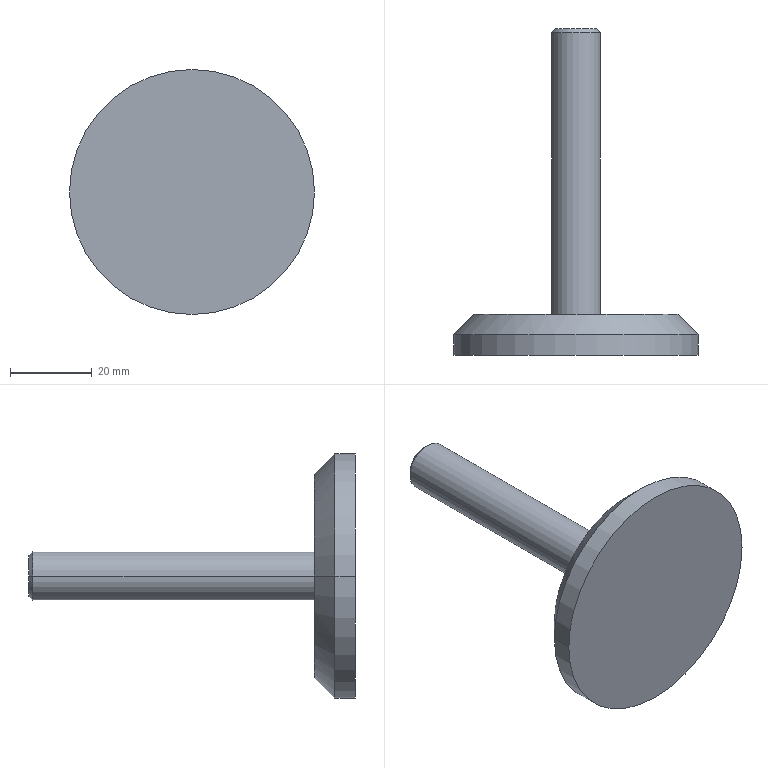Part | STEP file | Main support leg M12 for conveyor | 1 solid | 11 faces | box 60 x 80 x 60 mm | volume 33948 mm3 | cone 4 | cylinder 4 | plane 3 | commonest cylinder face diameters 12 x2 60 x2
STEP:
#1=CARTESIAN_POINT('',(-5.,80.,0.));
#2=VERTEX_POINT('',#1);
#3=CARTESIAN_POINT('',(5.,80.,0.));
#4=VERTEX_POINT('',#3);
#5=CARTESIAN_POINT('',(0.,80.,0.));
#6=DIRECTION('',(0.,1.,0.));
#7=DIRECTION('',(-1.,0.,0.));
#8=AXIS2_PLACEMENT_3D('',#5,#6,#7);
#9=CIRCLE('',#8,5.);
#10=EDGE_CURVE('',#2,#4,#9,.T.);
#11=ORIENTED_EDGE('',*,*,#10,.F.);
#12=CARTESIAN_POINT('',(-6.,79.,0.));
#13=VERTEX_POINT('',#12);
#14=CARTESIAN_POINT('',(-5.,80.,0.));
#15=DIRECTION('',(-0.7071,-0.7071,0.));
#16=VECTOR('',#15,1000.);
#17=LINE('',#14,#16);
#18=EDGE_CURVE('',#2,#13,#17,.T.);
#19=ORIENTED_EDGE('',*,*,#18,.T.);
#20=CARTESIAN_POINT('',(6.,79.,0.));
#21=VERTEX_POINT('',#20);
#22=CARTESIAN_POINT('',(0.,79.,0.));
#23=DIRECTION('',(0.,-1.,0.));
#24=DIRECTION('',(-1.,0.,0.));
#25=AXIS2_PLACEMENT_3D('',#22,#23,#24);
#26=CIRCLE('',#25,6.);
#27=EDGE_CURVE('',#21,#13,#26,.T.);
#28=ORIENTED_EDGE('',*,*,#27,.F.);
#29=CARTESIAN_POINT('',(5.,80.,0.));
#30=DIRECTION('',(0.7071,-0.7071,0.));
#31=VECTOR('',#30,1000.);
#32=LINE('',#29,#31);
#33=EDGE_CURVE('',#4,#21,#32,.T.);
#34=ORIENTED_EDGE('',*,*,#33,.F.);
#35=EDGE_LOOP('',(#11,#19,#28,#34));
#36=FACE_OUTER_BOUND('',#35,.T.);
#37=CARTESIAN_POINT('',(0.,80.,0.));
#38=DIRECTION('',(0.,-1.,0.));
#39=DIRECTION('',(1.,0.,0.));
#40=AXIS2_PLACEMENT_3D('',#37,#38,#39);
#41=CONICAL_SURFACE('',#40,5.,0.7854);
#42=ADVANCED_FACE('',(#36),#41,.T.);
#43=CARTESIAN_POINT('',(-6.,10.,0.));
#44=VERTEX_POINT('',#43);
#45=CARTESIAN_POINT('',(6.,10.,0.));
#46=VERTEX_POINT('',#45);
#47=CARTESIAN_POINT('',(0.,10.,0.));
#48=DIRECTION('',(0.,1.,0.));
#49=DIRECTION('',(-1.,0.,0.));
#50=AXIS2_PLACEMENT_3D('',#47,#48,#49);
#51=CIRCLE('',#50,6.);
#52=EDGE_CURVE('',#44,#46,#51,.T.);
#53=ORIENTED_EDGE('',*,*,#52,.T.);
#54=CARTESIAN_POINT('',(6.,80.,0.));
#55=DIRECTION('',(0.,1.,0.));
#56=VECTOR('',#55,1000.);
#57=LINE('',#54,#56);
#58=EDGE_CURVE('',#46,#21,#57,.T.);
#59=ORIENTED_EDGE('',*,*,#58,.T.);
#60=ORIENTED_EDGE('',*,*,#27,.T.);
#61=CARTESIAN_POINT('',(-6.,80.,0.));
#62=DIRECTION('',(0.,1.,0.));
#63=VECTOR('',#62,1000.);
#64=LINE('',#61,#63);
#65=EDGE_CURVE('',#44,#13,#64,.T.);
#66=ORIENTED_EDGE('',*,*,#65,.F.);
#67=EDGE_LOOP('',(#53,#59,#60,#66));
#68=FACE_OUTER_BOUND('',#67,.T.);
#69=CARTESIAN_POINT('',(0.,80.,0.));
#70=DIRECTION('',(0.,1.,0.));
#71=DIRECTION('',(-1.,0.,0.));
#72=AXIS2_PLACEMENT_3D('',#69,#70,#71);
#73=CYLINDRICAL_SURFACE('',#72,6.);
#74=ADVANCED_FACE('',(#68),#73,.T.);
#75=CARTESIAN_POINT('',(-25.,10.,0.));
#76=VERTEX_POINT('',#75);
#77=CARTESIAN_POINT('',(25.,10.,0.));
#78=VERTEX_POINT('',#77);
#79=CARTESIAN_POINT('',(0.,10.,0.));
#80=DIRECTION('',(0.,1.,0.));
#81=DIRECTION('',(-1.,0.,0.));
#82=AXIS2_PLACEMENT_3D('',#79,#80,#81);
#83=CIRCLE('',#82,25.);
#84=EDGE_CURVE('',#76,#78,#83,.T.);
#85=ORIENTED_EDGE('',*,*,#84,.F.);
#86=CARTESIAN_POINT('',(-30.,5.,0.));
#87=VERTEX_POINT('',#86);
#88=CARTESIAN_POINT('',(-25.,10.,0.));
#89=DIRECTION('',(-0.7071,-0.7071,0.));
#90=VECTOR('',#89,1000.);
#91=LINE('',#88,#90);
#92=EDGE_CURVE('',#76,#87,#91,.T.);
#93=ORIENTED_EDGE('',*,*,#92,.T.);
#94=CARTESIAN_POINT('',(30.,5.,0.));
#95=VERTEX_POINT('',#94);
#96=CARTESIAN_POINT('',(0.,5.,0.));
#97=DIRECTION('',(0.,1.,0.));
#98=DIRECTION('',(-1.,0.,0.));
#99=AXIS2_PLACEMENT_3D('',#96,#97,#98);
#100=CIRCLE('',#99,30.);
#101=EDGE_CURVE('',#87,#95,#100,.T.);
#102=ORIENTED_EDGE('',*,*,#101,.T.);
#103=CARTESIAN_POINT('',(25.,10.,0.));
#104=DIRECTION('',(0.7071,-0.7071,0.));
#105=VECTOR('',#104,1000.);
#106=LINE('',#103,#105);
#107=EDGE_CURVE('',#78,#95,#106,.T.);
#108=ORIENTED_EDGE('',*,*,#107,.F.);
#109=EDGE_LOOP('',(#85,#93,#102,#108));
#110=FACE_OUTER_BOUND('',#109,.T.);
#111=CARTESIAN_POINT('',(0.,10.,0.));
#112=DIRECTION('',(0.,-1.,0.));
#113=DIRECTION('',(1.,0.,0.));
#114=AXIS2_PLACEMENT_3D('',#111,#112,#113);
#115=CONICAL_SURFACE('',#114,25.,0.7854);
#116=ADVANCED_FACE('',(#110),#115,.T.);
#117=CARTESIAN_POINT('',(-30.,0.,0.));
#118=VERTEX_POINT('',#117);
#119=CARTESIAN_POINT('',(30.,0.,0.));
#120=VERTEX_POINT('',#119);
#121=CARTESIAN_POINT('',(0.,0.,0.));
#122=DIRECTION('',(0.,1.,0.));
#123=DIRECTION('',(-1.,0.,0.));
#124=AXIS2_PLACEMENT_3D('',#121,#122,#123);
#125=CIRCLE('',#124,30.);
#126=EDGE_CURVE('',#118,#120,#125,.T.);
#127=ORIENTED_EDGE('',*,*,#126,.T.);
#128=CARTESIAN_POINT('',(30.,80.,0.));
#129=DIRECTION('',(0.,1.,0.));
#130=VECTOR('',#129,1000.);
#131=LINE('',#128,#130);
#132=EDGE_CURVE('',#120,#95,#131,.T.);
#133=ORIENTED_EDGE('',*,*,#132,.T.);
#134=ORIENTED_EDGE('',*,*,#101,.F.);
#135=CARTESIAN_POINT('',(-30.,80.,0.));
#136=DIRECTION('',(0.,1.,0.));
#137=VECTOR('',#136,1000.);
#138=LINE('',#135,#137);
#139=EDGE_CURVE('',#118,#87,#138,.T.);
#140=ORIENTED_EDGE('',*,*,#139,.F.);
#141=EDGE_LOOP('',(#127,#133,#134,#140));
#142=FACE_OUTER_BOUND('',#141,.T.);
#143=CARTESIAN_POINT('',(0.,80.,0.));
#144=DIRECTION('',(0.,1.,0.));
#145=DIRECTION('',(-1.,0.,0.));
#146=AXIS2_PLACEMENT_3D('',#143,#144,#145);
#147=CYLINDRICAL_SURFACE('',#146,30.);
#148=ADVANCED_FACE('',(#142),#147,.T.);
#149=ORIENTED_EDGE('',*,*,#126,.F.);
#150=CARTESIAN_POINT('',(0.,0.,0.));
#151=DIRECTION('',(0.,1.,0.));
#152=DIRECTION('',(-1.,0.,0.));
#153=AXIS2_PLACEMENT_3D('',#150,#151,#152);
#154=CIRCLE('',#153,30.);
#155=EDGE_CURVE('',#120,#118,#154,.T.);
#156=ORIENTED_EDGE('',*,*,#155,.F.);
#157=EDGE_LOOP('',(#149,#156));
#158=FACE_OUTER_BOUND('',#157,.T.);
#159=CARTESIAN_POINT('',(0.,0.,0.));
#160=DIRECTION('',(0.,-1.,0.));
#161=DIRECTION('',(1.,0.,0.));
#162=AXIS2_PLACEMENT_3D('',#159,#160,#161);
#163=PLANE('',#162);
#164=ADVANCED_FACE('',(#158),#163,.T.);
#165=ORIENTED_EDGE('',*,*,#132,.F.);
#166=ORIENTED_EDGE('',*,*,#155,.T.);
#167=ORIENTED_EDGE('',*,*,#139,.T.);
#168=CARTESIAN_POINT('',(0.,5.,0.));
#169=DIRECTION('',(0.,1.,0.));
#170=DIRECTION('',(-1.,0.,0.));
#171=AXIS2_PLACEMENT_3D('',#168,#169,#170);
#172=CIRCLE('',#171,30.);
#173=EDGE_CURVE('',#95,#87,#172,.T.);
#174=ORIENTED_EDGE('',*,*,#173,.F.);
#175=EDGE_LOOP('',(#165,#166,#167,#174));
#176=FACE_OUTER_BOUND('',#175,.T.);
#177=CARTESIAN_POINT('',(0.,80.,0.));
#178=DIRECTION('',(0.,1.,0.));
#179=DIRECTION('',(-1.,0.,0.));
#180=AXIS2_PLACEMENT_3D('',#177,#178,#179);
#181=CYLINDRICAL_SURFACE('',#180,30.);
#182=ADVANCED_FACE('',(#176),#181,.T.);
#183=ORIENTED_EDGE('',*,*,#92,.F.);
#184=CARTESIAN_POINT('',(0.,10.,0.));
#185=DIRECTION('',(0.,1.,0.));
#186=DIRECTION('',(-1.,0.,0.));
#187=AXIS2_PLACEMENT_3D('',#184,#185,#186);
#188=CIRCLE('',#187,25.);
#189=EDGE_CURVE('',#78,#76,#188,.T.);
#190=ORIENTED_EDGE('',*,*,#189,.F.);
#191=ORIENTED_EDGE('',*,*,#107,.T.);
#192=ORIENTED_EDGE('',*,*,#173,.T.);
#193=EDGE_LOOP('',(#183,#190,#191,#192));
#194=FACE_OUTER_BOUND('',#193,.T.);
#195=CARTESIAN_POINT('',(0.,10.,0.));
#196=DIRECTION('',(0.,-1.,0.));
#197=DIRECTION('',(1.,0.,0.));
#198=AXIS2_PLACEMENT_3D('',#195,#196,#197);
#199=CONICAL_SURFACE('',#198,25.,0.7854);
#200=ADVANCED_FACE('',(#194),#199,.T.);
#201=ORIENTED_EDGE('',*,*,#189,.T.);
#202=ORIENTED_EDGE('',*,*,#84,.T.);
#203=EDGE_LOOP('',(#201,#202));
#204=FACE_OUTER_BOUND('',#203,.T.);
#205=ORIENTED_EDGE('',*,*,#52,.F.);
#206=CARTESIAN_POINT('',(0.,10.,0.));
#207=DIRECTION('',(0.,1.,0.));
#208=DIRECTION('',(-1.,0.,0.));
#209=AXIS2_PLACEMENT_3D('',#206,#207,#208);
#210=CIRCLE('',#209,6.);
#211=EDGE_CURVE('',#46,#44,#210,.T.);
#212=ORIENTED_EDGE('',*,*,#211,.F.);
#213=EDGE_LOOP('',(#205,#212));
#214=FACE_BOUND('',#213,.T.);
#215=CARTESIAN_POINT('',(-25.,10.,0.));
#216=DIRECTION('',(0.,1.,0.));
#217=DIRECTION('',(-1.,0.,0.));
#218=AXIS2_PLACEMENT_3D('',#215,#216,#217);
#219=PLANE('',#218);
#220=ADVANCED_FACE('',(#204,#214),#219,.T.);
#221=ORIENTED_EDGE('',*,*,#58,.F.);
#222=ORIENTED_EDGE('',*,*,#211,.T.);
#223=ORIENTED_EDGE('',*,*,#65,.T.);
#224=CARTESIAN_POINT('',(0.,79.,0.));
#225=DIRECTION('',(0.,-1.,0.));
#226=DIRECTION('',(-1.,0.,0.));
#227=AXIS2_PLACEMENT_3D('',#224,#225,#226);
#228=CIRCLE('',#227,6.);
#229=EDGE_CURVE('',#13,#21,#228,.T.);
#230=ORIENTED_EDGE('',*,*,#229,.T.);
#231=EDGE_LOOP('',(#221,#222,#223,#230));
#232=FACE_OUTER_BOUND('',#231,.T.);
#233=CARTESIAN_POINT('',(0.,80.,0.));
#234=DIRECTION('',(0.,1.,0.));
#235=DIRECTION('',(-1.,0.,0.));
#236=AXIS2_PLACEMENT_3D('',#233,#234,#235);
#237=CYLINDRICAL_SURFACE('',#236,6.);
#238=ADVANCED_FACE('',(#232),#237,.T.);
#239=CARTESIAN_POINT('',(0.,80.,0.));
#240=DIRECTION('',(0.,1.,0.));
#241=DIRECTION('',(-1.,0.,0.));
#242=AXIS2_PLACEMENT_3D('',#239,#240,#241);
#243=CIRCLE('',#242,5.);
#244=EDGE_CURVE('',#4,#2,#243,.T.);
#245=ORIENTED_EDGE('',*,*,#244,.T.);
#246=ORIENTED_EDGE('',*,*,#10,.T.);
#247=EDGE_LOOP('',(#245,#246));
#248=FACE_OUTER_BOUND('',#247,.T.);
#249=CARTESIAN_POINT('',(-6.,80.,0.));
#250=DIRECTION('',(0.,1.,0.));
#251=DIRECTION('',(-1.,0.,0.));
#252=AXIS2_PLACEMENT_3D('',#249,#250,#251);
#253=PLANE('',#252);
#254=ADVANCED_FACE('',(#248),#253,.T.);
#255=ORIENTED_EDGE('',*,*,#18,.F.);
#256=ORIENTED_EDGE('',*,*,#244,.F.);
#257=ORIENTED_EDGE('',*,*,#33,.T.);
#258=ORIENTED_EDGE('',*,*,#229,.F.);
#259=EDGE_LOOP('',(#255,#256,#257,#258));
#260=FACE_OUTER_BOUND('',#259,.T.);
#261=CARTESIAN_POINT('',(0.,80.,0.));
#262=DIRECTION('',(0.,-1.,0.));
#263=DIRECTION('',(1.,0.,0.));
#264=AXIS2_PLACEMENT_3D('',#261,#262,#263);
#265=CONICAL_SURFACE('',#264,5.,0.7854);
#266=ADVANCED_FACE('',(#260),#265,.T.);
#267=CLOSED_SHELL('',(#42,#74,#116,#148,#164,#182,#200,#220,#238,#254,#266));
#268=MANIFOLD_SOLID_BREP('',#267);
#269=CARTESIAN_POINT('',(0.,0.,0.));
#270=DIRECTION('',(0.,0.,1.));
#271=DIRECTION('',(1.,0.,0.));
#272=AXIS2_PLACEMENT_3D('',#269,#270,#271);
#273=(LENGTH_UNIT()NAMED_UNIT(*)SI_UNIT(.MILLI.,.METRE.));
#274=UNCERTAINTY_MEASURE_WITH_UNIT(LENGTH_MEASURE(0.00001),#273,'','');
#275=(NAMED_UNIT(*)PLANE_ANGLE_UNIT()SI_UNIT($,.RADIAN.));
#276=(NAMED_UNIT(*)SI_UNIT($,.STERADIAN.)SOLID_ANGLE_UNIT());
#277=(GEOMETRIC_REPRESENTATION_CONTEXT(3)GLOBAL_UNCERTAINTY_ASSIGNED_CONTEXT((#274))GLOBAL_UNIT_ASSIGNED_CONTEXT((#273,#275,#276))REPRESENTATION_CONTEXT('',''));
#278=ADVANCED_BREP_SHAPE_REPRESENTATION('',(#268,#272),#277);